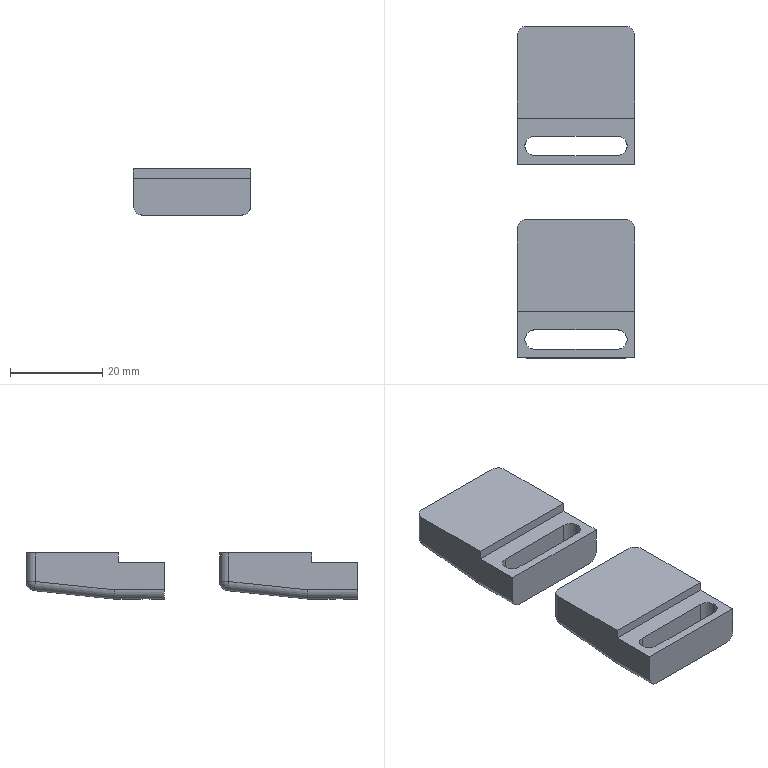NC program | NX | posted with a generic post | part box 25.5 x 72 x 10 mm
Lines 86 to 1188 of 60534:
(FIXED_CONTOUR , TOOL : D4R0.5)
N164 T16 M6
N166 G54
N168 G17 G0 G90 X3.812 Y-11.316 B0. C0. S9500 M3
N170 G43 Z30. H16
N172 Z1.2
N174 G94 G1 Z-4.301 F1000.
N176 G3 X4.012 Y-10.97 R0.4
N178 G1 Y-10.947 Z-4.21 F2500.
N180 X4.01 Y-10.907 Z-4.201
N182 X4.005 Y-10.808
N184 X4.003 Y-1.71
N186 X4.007 Y-1.464
N188 X4.012 Y-1.388 Z-4.189
N190 Y-1.294 Z-4.213
N192 Y-1.388 Z-4.189
N194 X4.011 Y-1.413 Z-4.193
N196 Y-1.541 Z-4.157
N198 Y-1.937 Z-4.103
N200 Y-2.334 Z-4.104
N202 Y-2.755 Z-4.101
N204 Y-7.911 Z-4.121
N206 Y-9.101 Z-4.128
N208 Y-10.709 Z-4.126
N210 Y-10.75 Z-4.132
N212 Y-10.808 Z-4.135
N214 Y-10.907 Z-4.19
N216 Y-10.919 Z-4.204
N218 X4.012 Y-10.947 Z-4.21
N220 Y-10.97 Z-4.301
N222 X4.018 Y-11.032
N224 Y-11.009 Z-4.209
N226 Y-10.907 Z-4.095
N228 Y-10.808 Z-4.039
N230 Y-10.789 Z-4.038
N232 Y-10.709 Z-4.026
N234 Y-8.924 Z-4.028
N236 Y-4.165 Z-4.013
N238 Y-2.926 Z-4.011
N240 Y-2.578 Z-4.02
N242 Y-2.084 Z-4.018
N244 Y-1.687 Z-4.072
N246 Y-1.388 Z-4.157
N248 Y-1.264 Z-4.189
N250 X4.023 Y-1.237 Z-4.167
N252 X4.028 Y-1.224 Z-4.157
N254 Y-1.388 Z-4.114
N256 Y-1.478 Z-4.086
N258 Y-1.785 Z-3.999
N260 Y-1.875 Z-3.979
N262 Y-2.181 Z-3.937
N264 Y-2.271 Z-3.935
N266 Y-2.703 Z-3.936
N268 Y-3.144 Z-3.94
N270 Y-7.903 Z-3.945
N272 Y-9.152 Z-3.947
N274 Y-10.709 Z-3.944
N276 Y-10.808 Z-3.95
N278 Y-10.907 Z-3.982
N280 Y-10.921 Z-3.991
N282 Y-10.942 Z-4.013
N284 Y-11.116 Z-4.208
N286 Y-11.139 Z-4.301
N288 X4.037 Y-11.246
N290 Y-11.223 Z-4.206
N292 Y-11.149 Z-4.123
N294 Y-11. Z-3.973
N296 Y-10.907 Z-3.912
N298 Y-10.808 Z-3.88
N300 Y-10.709 Z-3.874
N302 Y-4.958 Z-3.886
N304 Y-2.46 Z-3.878
N306 Y-2.181 Z-3.885
N308 Y-2.064 Z-3.901
N310 Y-1.785 Z-3.964
N312 Y-1.667 Z-3.998
N314 Y-1.388 Z-4.083
N316 Y-1.195 Z-4.136
N318 X4.049 Y-1.164 Z-4.113
N320 Y-1.346 Z-4.063
N322 Y-1.444 Z-4.032
N324 Y-1.841 Z-3.911
N326 Y-2.21 Z-3.828
N328 Y-2.238 Z-3.825
N330 Y-2.656 Z-3.816
N332 Y-2.975 Z-3.822
N334 Y-5.354 Z-3.827
N336 Y-7.338 Z-3.825
N338 Y-8.657 Z-3.824
N340 Y-10.709 Z-3.819
N342 Y-10.808 Z-3.821
N344 Y-10.907 Z-3.843
N346 Y-10.984 Z-3.877
N348 Y-11.097 Z-3.951
N350 Y-11.304 Z-4.159
N352 Y-11.328 Z-4.205
N354 Y-11.339 Z-4.301
N356 X4.063 Y-11.411
N358 Y-11.4 Z-4.206
N360 Y-11.38 Z-4.161
N362 Y-11.304 Z-4.019
N364 Y-11.211 Z-3.925
N366 Y-11.16 Z-3.891
N368 Y-10.907 Z-3.779
N370 Y-10.808 Z-3.758
N372 Y-10.709 Z-3.755
N374 Y-8.021 Z-3.763
N376 Y-6.257 Z-3.758
N378 Y-3.481 Z-3.756
N380 Y-2.975 Z-3.755
N382 Y-2.844 Z-3.753
N384 Y-2.578 Z-3.755
N386 Y-2.373 Z-3.761
N388 Y-2.277 Z-3.769
N390 Y-2.181 Z-3.788
N392 Y-1.976 Z-3.834
N394 Y-1.58 Z-3.955
N396 Y-1.388 Z-4.019
N398 Y-1.245 Z-4.063
N400 Y-1.135 Z-4.094
N402 X4.079 Y-1.1 Z-4.07
N404 Y-1.388 Z-3.981
N406 Y-1.785 Z-3.85
N408 Y-2.135 Z-3.745
N410 Y-2.357 Z-3.699
N412 Y-2.532 Z-3.684
N414 Y-2.744 Z-3.681
N416 Y-2.975 Z-3.686
N418 Y-6.978 Z-3.691
N420 Y-8.131 Z-3.696
N422 Y-10.709 Z-3.688
N424 Y-10.816 Z-3.692
N426 Y-10.916 Z-3.709
N428 Y-10.936 Z-3.716
N430 Y-11.304 Z-3.878
N432 Y-11.333 Z-3.909
N434 Y-11.447 Z-4.122
N436 Y-11.485 Z-4.207
N438 Y-11.496 Z-4.301
N440 X4.098 Y-11.595
N442 Y-11.584 Z-4.207
N444 Y-11.525 Z-4.077
N446 Y-11.446 Z-3.929
N448 Y-11.304 Z-3.783
N450 Y-11.217 Z-3.744
N452 Y-11.003 Z-3.67
N454 Y-10.907 Z-3.642
N456 Y-10.808 Z-3.626
N458 Y-10.709 Z-3.624
N460 Y-8.131 Z-3.63
N462 Y-6.4 Z-3.626
N464 Y-2.975 Z-3.621
N466 Y-2.674 Z-3.615
N468 Y-2.578 Z-3.619
N470 Y-2.436 Z-3.631
N472 Y-2.295 Z-3.66
N474 Y-2.181 Z-3.688
N476 Y-1.898 Z-3.773
N478 Y-1.785 Z-3.814
N480 Y-1.445 Z-3.927
N482 Y-1.388 Z-3.949
N484 Y-1.064 Z-4.049
N486 X4.117 Y-1.03 Z-4.03
N488 Y-1.388 Z-3.919
N490 Y-1.521 Z-3.869
N492 Y-1.785 Z-3.781
N494 Y-2.05 Z-3.686
N496 Y-2.181 Z-3.646
N498 Y-2.446 Z-3.581
N500 Y-2.512 Z-3.568
N502 Y-2.578 Z-3.562
N504 Y-2.802 Z-3.553
N506 Y-2.975 Z-3.557
N508 Y-8.527 Z-3.563
N510 Y-10.709 Z-3.559
N512 Y-10.808 Z-3.562
N514 Y-10.907 Z-3.577
N516 Y-11.09 Z-3.632
N518 Y-11.304 Z-3.705
N520 Y-11.357 Z-3.742
N522 Y-11.395 Z-3.772
N524 Y-11.445 Z-3.832
N526 Y-11.559 Z-3.949
N528 Y-11.603 Z-4.031
N530 Y-11.683 Z-4.208
N532 Y-11.694 Z-4.301
N534 X4.138 Y-11.765
N536 Y-11.758 Z-4.212
N538 Y-11.7 Z-4.011
N540 Y-11.682 Z-3.971
N542 Y-11.667 Z-3.956
N544 Y-11.538 Z-3.803
N546 Y-11.441 Z-3.724
N548 Y-11.304 Z-3.63
N550 Y-11.185 Z-3.589
N552 Y-10.907 Z-3.507
N554 Y-10.808 Z-3.492
N556 Y-10.709 Z-3.489
N558 Y-6.12 Z-3.492
N560 Y-2.941 Z-3.486
N562 Y-2.598 Z-3.501
N564 Y-2.578 Z-3.504
N566 Y-2.214 Z-3.594
N568 Y-2.149 Z-3.615
N570 Y-1.785 Z-3.746
N572 Y-1.603 Z-3.806
N574 Y-1.388 Z-3.888
N576 Y-0.992 Z-4.009
N578 X4.16 Y-0.953 Z-3.99
N580 Y-0.992 Z-3.981
N582 Y-1.176 Z-3.918
N584 Y-1.388 Z-3.853
N586 Y-1.692 Z-3.738
N588 Y-1.785 Z-3.707
N590 Y-2.181 Z-3.563
N592 Y-2.393 Z-3.502
N594 Y-2.578 Z-3.456
N596 Y-2.711 Z-3.439
N598 Y-2.975 Z-3.426
N600 Y-6.148 Z-3.43
N602 Y-10.709 Z-3.429
N604 Y-10.808 Z-3.431
N606 Y-10.907 Z-3.443
N608 Y-11.227 Z-3.525
N610 Y-11.304 Z-3.549
N612 Y-11.532 Z-3.705
N614 Y-11.694 Z-3.837
N616 Y-11.7 Z-3.845
N618 Y-11.764 Z-3.975
N620 Y-11.834 Z-4.216
N622 Y-11.841 Z-4.301
N624 X4.189 Y-11.936
N626 Y-11.929 Z-4.221
N628 Y-11.859 Z-3.975
N630 Y-11.79 Z-3.837
N632 Y-11.768 Z-3.805
N634 Y-11.7 Z-3.723
N636 Y-11.648 Z-3.68
N638 Y-11.565 Z-3.624
N640 Y-11.387 Z-3.511
N642 Y-11.304 Z-3.466
N644 Y-11.107 Z-3.422
N646 Y-10.907 Z-3.37
N648 Y-10.808 Z-3.359
N650 Y-10.709 Z-3.357
N652 Y-8.392 Z-3.359
N654 Y-2.975 Z-3.355
N656 Y-2.854 Z-3.361
N658 Y-2.589 Z-3.395
N660 Y-2.181 Z-3.515
N662 Y-1.785 Z-3.661
N664 Y-1.388 Z-3.812
N666 Y-0.992 Z-3.948
N668 Y-0.904 Z-3.967
N670 X4.204 Y-0.879 Z-3.955
N672 X4.218 Y-0.862 Z-3.949
N674 Y-0.992 Z-3.915
N676 Y-1.388 Z-3.78
N678 Y-1.523 Z-3.724
N680 Y-1.785 Z-3.625
N682 Y-1.92 Z-3.57
N684 Y-2.181 Z-3.474
N686 Y-2.317 Z-3.428
N688 Y-2.578 Z-3.352
N690 Y-2.646 Z-3.334
N692 Y-2.713 Z-3.322
N694 Y-2.975 Z-3.286
N696 Y-7.734 Z-3.288
N698 Y-8.924 Z-3.29
N700 Y-10.722 Z-3.286
N702 Y-10.808 Z-3.288
N704 Y-10.916 Z-3.3
N706 Y-11.304 Z-3.386
N708 Y-11.482 Z-3.483
N710 Y-11.7 Z-3.621
N712 Y-11.738 Z-3.65
N714 Y-11.838 Z-3.77
N716 Y-11.883 Z-3.836
N718 Y-11.953 Z-3.975
N720 Y-12.025 Z-4.227
N722 Y-12.032 Z-4.301
N724 X4.237 Y-12.097 Z-4.3
N726 X4.248 Y-12.126 Z-4.301
N728 Y-12.122 Z-4.236
N730 Y-12.115 Z-4.197
N732 Y-12.052 Z-3.975
N734 Y-11.981 Z-3.835
N736 Y-11.911 Z-3.733
N738 Y-11.812 Z-3.615
N740 Y-11.7 Z-3.528
N742 Y-11.582 Z-3.453
N744 Y-11.384 Z-3.345
N746 Y-11.304 Z-3.315
N748 Y-11.224 Z-3.292
N750 Y-11.003 Z-3.244
N752 Y-10.907 Z-3.234
N754 Y-10.806 Z-3.22
N756 Y-10.709 Z-3.223
N758 Y-8.332 Z-3.224
N760 Y-5.153 Z-3.223
N762 Y-3.567
N764 Y-3.17 Z-3.222
N766 Y-2.975 Z-3.227
N768 Y-2.833 Z-3.246
N770 Y-2.705 Z-3.27
N772 Y-2.578 Z-3.303
N774 Y-2.436 Z-3.344
N776 Y-2.181 Z-3.432
N778 Y-2.04 Z-3.483
N780 Y-1.785 Z-3.587
N782 Y-1.643 Z-3.641
N784 Y-1.388 Z-3.746
N786 Y-1.19 Z-3.813
N788 Y-0.992 Z-3.887
N790 Y-0.884 Z-3.921
N792 Y-0.823 Z-3.936
N794 X4.278 Y-0.782 Z-3.924
N796 Y-0.992 Z-3.858
N798 Y-1.388 Z-3.712
N800 Y-2.161 Z-3.396
N802 Y-2.578 Z-3.253
N804 Y-2.766 Z-3.205
N806 Y-2.975 Z-3.167
N808 Y-3.371 Z-3.158
N810 Y-4.165 Z-3.161
N812 Y-8.131 Z-3.158
N814 Y-10.724
N816 Y-10.808 Z-3.159
N818 Y-10.907 Z-3.169
N820 Y-11.09 Z-3.188
N822 Y-11.123 Z-3.195
N824 Y-11.304 Z-3.247
N826 Y-11.485 Z-3.313
N828 Y-11.7 Z-3.434
N830 Y-11.886 Z-3.579
N832 Y-11.985 Z-3.695
N834 Y-12.08 Z-3.833
N836 Y-12.097 Z-3.867
N838 Y-12.169 Z-4.037
N840 Y-12.181 Z-4.077
N842 Y-12.209 Z-4.264
N844 Z-4.301
N846 X4.317 Y-12.3
N848 Y-12.299 Z-4.254
N850 Y-12.266 Z-4.046
N852 Y-12.233 Z-3.962
N854 Y-12.183 Z-3.848
N856 Y-12.097 Z-3.696
N858 Y-12.066 Z-3.651
N860 Y-12.035 Z-3.614
N862 Y-11.967 Z-3.544
N864 Y-11.768 Z-3.39
N866 Y-11.7 Z-3.342
N868 Y-11.57 Z-3.269
N870 Y-11.372 Z-3.198
N872 Y-11.304 Z-3.171
N874 Y-11.174 Z-3.134
N876 Y-11.037 Z-3.111
N878 Y-10.842 Z-3.091
N880 Y-10.511 Z-3.088
N882 Y-4.822
N884 Y-3.768
N886 Y-3.371 Z-3.087
N888 Y-3.111 Z-3.094
N890 Y-2.975 Z-3.106
N892 Y-2.844 Z-3.13
N894 Y-2.578 Z-3.2
N896 Y-2.317 Z-3.29
N898 Y-2.181 Z-3.342
N900 Y-1.921 Z-3.448
N902 Y-1.785 Z-3.507
N904 Y-1.524 Z-3.614
N906 Y-1.388 Z-3.674
N908 Y-1.128 Z-3.771
N910 Y-0.992 Z-3.826
N912 Y-0.73 Z-3.91
N914 X4.358 Y-0.677 Z-3.897
N916 Y-0.992 Z-3.794
N918 Y-1.289 Z-3.674
N920 Y-1.388 Z-3.637
N922 Y-1.686 Z-3.506
N924 Y-1.785 Z-3.465
N926 Y-2.083 Z-3.335
N928 Y-2.181 Z-3.295
N930 Y-2.479 Z-3.181
N932 Y-2.578 Z-3.147
N934 Y-2.925 Z-3.055
N936 Y-2.975 Z-3.045
N938 Y-3.272 Z-3.018
N940 Y-3.371 Z-3.016
N942 Y-10.511
N944 Y-10.882 Z-3.023
N946 Y-10.957 Z-3.03
N948 Y-11.254 Z-3.081
N950 Y-11.304 Z-3.095
N952 Y-11.453 Z-3.154
N954 Y-11.651 Z-3.223
N956 Y-11.7 Z-3.251
N958 Y-11.849 Z-3.357
N960 Y-12.048 Z-3.509
N962 Y-12.097 Z-3.56
N964 Y-12.144 Z-3.62
N966 Y-12.167 Z-3.653
N968 Y-12.19 Z-3.696
N970 Y-12.286 Z-3.866
N972 Y-12.336 Z-3.983
N974 Y-12.354 Z-4.034
N976 Y-12.389 Z-4.247
N978 Y-12.392 Z-4.301
N980 X4.398 Y-12.483
N982 Y-12.477 Z-4.228
N984 Y-12.441 Z-4.022
N986 Y-12.406 Z-3.923
N988 Y-12.389 Z-3.884
N990 Y-12.34 Z-3.798
N992 Y-12.281 Z-3.685
N994 Y-12.221 Z-3.598
N996 Y-12.124 Z-3.479
N998 Y-12.097 Z-3.451
N1000 Y-11.93 Z-3.323
N1002 Y-11.763 Z-3.204
N1004 Y-11.7 Z-3.167
N1006 Y-11.534 Z-3.11
N1008 Y-11.367 Z-3.044
N1010 Y-11.304 Z-3.024
N1012 Y-10.97 Z-2.967
N1014 Y-10.907 Z-2.957
N1016 Y-10.511 Z-2.949
N1018 Y-3.371
N1020 Y-3.006 Z-2.983
N1022 Y-2.975 Z-2.989
N1024 Y-2.61 Z-3.087
N1026 Y-2.578 Z-3.098
N1028 Y-2.244 Z-3.225
N1030 Y-2.181 Z-3.251
N1032 Y-1.848 Z-3.396
N1034 Y-1.388 Z-3.602
N1036 Y-1.054 Z-3.736
N1038 Y-0.992 Z-3.763
N1040 Y-0.66 Z-3.875
N1042 Y-0.625 Z-3.885
N1044 X4.441 Y-0.575 Z-3.876
N1046 Y-0.676 Z-3.845
N1048 Y-0.816 Z-3.798
N1050 Y-0.992 Z-3.734
N1052 Y-1.223 Z-3.635
N1054 Y-1.388 Z-3.569
N1056 Y-1.619 Z-3.461
N1058 Y-1.785 Z-3.388
N1060 Y-2.016 Z-3.281
N1062 Y-2.181 Z-3.209
N1064 Y-2.412 Z-3.114
N1066 Y-2.578 Z-3.051
N1068 Y-2.694 Z-3.012
N1070 Y-2.975 Z-2.937
N1072 Y-3.09 Z-2.914
N1074 Y-3.371 Z-2.888
N1076 Y-10.511
N1078 Y-10.907 Z-2.895
N1080 Y-11.023 Z-2.915
N1082 Y-11.138 Z-2.929
N1084 Y-11.304 Z-2.958
N1086 Y-11.419 Z-2.997
N1088 Y-11.535 Z-3.031
N1090 Y-11.618 Z-3.064
N1092 Y-11.7 Z-3.093
N1094 Y-11.816 Z-3.159
N1096 Y-11.931 Z-3.229
N1098 Y-12.014 Z-3.288
N1100 Y-12.097 Z-3.352
N1102 Y-12.197 Z-3.454
N1104 Y-12.24 Z-3.5
N1106 Y-12.3 Z-3.576
N1108 Y-12.399 Z-3.718
N1110 Y-12.495 Z-3.902
N1112 Y-12.526 Z-4.004
N1114 Y-12.548 Z-4.159
N1116 Y-12.562 Z-4.232
N1118 Y-12.566 Z-4.301
N1120 X4.485 Y-12.652
N1122 Y-12.648 Z-4.223
N1124 Y-12.616 Z-4.059
N1126 Y-12.604 Z-3.979
N1128 Y-12.582 Z-3.916
N1130 Y-12.567 Z-3.865
N1132 Y-12.519 Z-3.753
N1134 Y-12.494 Z-3.71
N1136 Y-12.384 Z-3.552
N1138 Y-12.35 Z-3.509
N1140 Y-12.274 Z-3.427
N1142 Y-12.097 Z-3.249
N1144 Y-11.904 Z-3.132
N1146 Y-11.7 Z-3.015
N1148 Y-11.508 Z-2.958
N1150 Y-11.304 Z-2.889
N1152 Y-11.111 Z-2.866
N1154 Y-10.907 Z-2.831
N1156 Y-10.511 Z-2.823
N1158 Y-5.349 Z-2.826
N1160 Y-3.768 Z-2.824
N1162 Y-3.371 Z-2.825
N1164 Y-3.173 Z-2.844
N1166 Y-2.978 Z-2.882
N1168 Y-2.779 Z-2.935
N1170 Y-2.581 Z-3.001
N1172 Y-2.187 Z-3.162
N1174 Y-1.382 Z-3.537
N1176 Y-0.992 Z-3.705
N1178 Y-0.595 Z-3.845
N1180 Y-0.524 Z-3.867
N1182 X4.532 Y-0.473 Z-3.862
N1184 Y-0.595 Z-3.823
N1186 Y-0.694 Z-3.783
N1188 Y-0.992 Z-3.678
N1190 Y-1.289 Z-3.55
N1192 Y-1.388 Z-3.503
N1194 Y-1.487 Z-3.453
N1196 Y-1.785 Z-3.314
N1198 Y-1.884 Z-3.263
N1200 Y-2.28 Z-3.081
N1202 Y-2.578 Z-2.959
N1204 Y-2.627 Z-2.941
N1206 Y-2.826 Z-2.875
N1208 Y-3.024 Z-2.824
N1210 Y-3.173 Z-2.795
N1212 Y-3.272 Z-2.777
N1214 Y-3.371 Z-2.768
N1216 Y-8.652
N1218 Y-10.609
N1220 Y-10.907 Z-2.774
N1222 Y-10.957 Z-2.778
N1224 Y-11.105 Z-2.796
N1226 Y-11.204 Z-2.813
N1228 Y-11.304 Z-2.825
N1230 Y-11.502 Z-2.882
N1232 Y-11.601 Z-2.916
N1234 Y-11.7 Z-2.946
N1236 Y-11.898 Z-3.046
N1238 Y-11.998 Z-3.103
N1240 Y-12.097 Z-3.163
N1242 Y-12.196 Z-3.243
N1244 Y-12.248 Z-3.291
N1246 Y-12.355 Z-3.399
N1248 Y-12.472 Z-3.527
N1250 Y-12.494 Z-3.558
N1252 Y-12.572 Z-3.682
N1254 Y-12.627 Z-3.789
N1256 Y-12.643 Z-3.826
N1258 Y-12.688 Z-3.954
N1260 Y-12.733 Z-4.218
N1262 Y-12.737 Z-4.301
N1264 X4.582 Y-12.82
N1266 Y-12.817 Z-4.219
N1268 Y-12.771 Z-3.952
N1270 Y-12.725 Z-3.807
N1272 Y-12.667 Z-3.68
N1274 Y-12.639 Z-3.628
N1276 Y-12.613 Z-3.586
N1278 Y-12.494 Z-3.425
N1280 Y-12.401 Z-3.328
N1282 Y-12.296 Z-3.232
N1284 Y-12.097 Z-3.072
N1286 Y-11.8 Z-2.92
N1288 Y-11.7 Z-2.872
N1290 Y-11.303 Z-2.757
N1292 Y-11.007 Z-2.72
N1294 Y-10.907 Z-2.714
N1296 Y-10.511 Z-2.707
N1298 Y-3.371 Z-2.708
N1300 Y-3.173 Z-2.742
N1302 Y-3.074 Z-2.761
N1304 Y-2.975 Z-2.785
N1306 Y-2.876 Z-2.812
N1308 Y-2.677 Z-2.876
N1310 Y-2.578 Z-2.913
N1312 Y-2.38 Z-2.994
N1314 Y-2.181 Z-3.083
N1316 Y-1.984 Z-3.175
N1318 Y-1.785 Z-3.276
N1320 Y-1.587 Z-3.368
N1322 Y-1.388 Z-3.47
N1324 Y-1.189 Z-3.565
N1326 Y-0.992 Z-3.649
N1328 Y-0.794 Z-3.719
N1330 Y-0.595 Z-3.799
N1332 Y-0.419 Z-3.857
N1334 X4.634 Y-0.367 Z-3.85
N1336 Y-0.595 Z-3.775
N1338 Y-0.897 Z-3.653
N1340 Y-0.992 Z-3.62
N1342 Y-1.086 Z-3.579
N1344 Y-1.388 Z-3.436
N1346 Y-1.69 Z-3.281
N1348 Y-1.785 Z-3.237
N1350 Y-2.087 Z-3.083
N1352 Y-2.483 Z-2.904
N1354 Y-2.578 Z-2.865
N1356 Y-2.729 Z-2.809
N1358 Y-2.927 Z-2.746
N1360 Y-3.126 Z-2.697
N1362 Y-3.371 Z-2.653
N1364 Y-3.578 Z-2.645
N1366 Y-10.511
N1368 Y-10.907 Z-2.651
N1370 Y-11.058 Z-2.661
N1372 Y-11.2 Z-2.678
N1374 Y-11.304 Z-2.695
N1376 Y-11.407 Z-2.719
N1378 Y-11.7 Z-2.804
N1380 Y-11.804 Z-2.845
N1382 Y-12.097 Z-2.993
N1384 Y-12.201 Z-3.061
N1386 Y-12.399 Z-3.221
N1388 Y-12.494 Z-3.307
N1390 Y-12.532 Z-3.35
N1392 Y-12.674 Z-3.538
N1394 Y-12.717 Z-3.605
N1396 Y-12.811 Z-3.807
N1398 Y-12.857 Z-3.952
N1400 Y-12.899 Z-4.196
N1402 Y-12.902 Z-4.225
N1404 Y-12.906 Z-4.301
N1406 X4.683 Y-12.984 Z-4.3
N1408 Y-12.982 Z-4.249
N1410 Y-12.96 Z-4.041
N1412 Y-12.938 Z-3.954
N1414 Y-12.89 Z-3.799
N1416 Y-12.796 Z-3.599
N1418 Y-12.697 Z-3.445
N1420 Y-12.622 Z-3.346
N1422 Y-12.494 Z-3.207
N1424 Y-12.3 Z-3.051
N1426 Y-12.097 Z-2.917
N1428 Y-11.903 Z-2.82
N1430 Y-11.7 Z-2.74
N1432 Y-11.504 Z-2.682
N1434 Y-11.304 Z-2.636
N1436 Y-11.103 Z-2.604
N1438 Y-10.907 Z-2.591
N1440 Y-10.506 Z-2.586
N1442 Y-3.768 Z-2.585
N1444 Y-3.371 Z-2.601
N1446 Y-3.175 Z-2.635
N1448 Y-2.975 Z-2.683
N1450 Y-2.779 Z-2.745
N1452 Y-2.578 Z-2.819
N1454 Y-2.181 Z-2.997
N1456 Y-1.388 Z-3.403
N1458 Y-0.992 Z-3.592
N1460 Y-0.595 Z-3.752
N1462 Y-0.32 Z-3.843
N1464 X4.739 Y-0.27 Z-3.839
N1466 Y-0.537 Z-3.752
N1468 Y-0.595 Z-3.731
N1470 Y-0.711 Z-3.679
N1472 Y-0.992 Z-3.566
N1474 Y-1.108 Z-3.506
N1476 Y-1.388 Z-3.373
N1478 Y-1.504 Z-3.308
N1480 Y-1.785 Z-3.164
N1482 Y-1.901 Z-3.1
N1484 Y-2.181 Z-2.958
N1486 Y-2.298 Z-2.902
N1488 Y-2.578 Z-2.776
N1490 Y-2.834 Z-2.682
N1492 Y-2.975 Z-2.638
N1494 Y-3.231 Z-2.577
N1496 Y-3.371 Z-2.553
N1498 Y-3.487 Z-2.544
N1500 Y-3.768 Z-2.533
N1502 Y-6.941
N1504 Y-10.511
N1506 Y-10.907 Z-2.538
N1508 Y-11.047 Z-2.547
N1510 Y-11.164 Z-2.558
N1512 Y-11.304 Z-2.58
N1514 Y-11.56 Z-2.639
N1516 Y-11.7 Z-2.68
N1518 Y-11.817 Z-2.723
N1520 Y-12.015 Z-2.801
N1522 Y-12.097 Z-2.843
N1524 Y-12.353 Z-3.009
N1526 Y-12.412 Z-3.049
N1528 Y-12.494 Z-3.115
N1530 Y-12.61 Z-3.234
N1532 Y-12.698 Z-3.33
N1534 Y-12.808 Z-3.477
N1536 Y-12.89 Z-3.607
N1538 Y-12.903 Z-3.632
N1540 Y-12.975 Z-3.826
N1542 Y-13.01 Z-3.941
N1544 Y-13.034 Z-4.034
N1546 Y-13.057 Z-4.247
N1548 Y-13.059 Z-4.301
N1550 X4.799 Y-13.139
N1552 Y-13.137 Z-4.244
N1554 Y-13.112 Z-4.026
N1556 Y-13.088 Z-3.928
N1558 Y-13.062 Z-3.845
N1560 Y-12.993 Z-3.656
N1562 Y-12.909 Z-3.49
N1564 Y-12.89 Z-3.461
N1566 Y-12.779 Z-3.313
N1568 Y-12.65 Z-3.176
N1570 Y-12.518 Z-3.044
N1572 Y-12.494 Z-3.022
N1574 Y-12.332 Z-2.914
N1576 Y-12.17 Z-2.81
N1578 Y-12.097 Z-2.767
N1580 Y-11.935 Z-2.704
N1582 Y-11.7 Z-2.617
N1584 Y-11.62 Z-2.593
N1586 Y-11.304 Z-2.521
N1588 Y-11.223 Z-2.508
N1590 Y-10.988 Z-2.486
N1592 Y-10.907 Z-2.481
N1594 Y-10.511 Z-2.476
N1596 Y-6.148 Z-2.477
N1598 Y-4.796 Z-2.478
N1600 Y-3.768 Z-2.476
N1602 Y-3.606 Z-2.483
N1604 Y-3.371 Z-2.501
N1606 Y-3.29 Z-2.515
N1608 Y-2.975 Z-2.59
N1610 Y-2.894 Z-2.615
N1612 Y-2.578 Z-2.73
N1614 Y-2.416 Z-2.803
N1616 Y-2.181 Z-2.916
N1618 Y-2.02 Z-2.998
N1620 Y-1.785 Z-3.126
N1622 Y-1.623 Z-3.209
N1624 Y-1.388 Z-3.34
N1626 Y-1.226 Z-3.417
N1628 Y-0.992 Z-3.538
N1630 Y-0.83 Z-3.603
N1632 Y-0.595 Z-3.709
N1634 Y-0.477 Z-3.752
N1636 Y-0.216 Z-3.836
N1638 X4.858 Y-0.172 Z-3.832
N1640 Y-0.418 Z-3.752
N1642 Y-0.595 Z-3.686
N1644 Y-0.949 Z-3.528
N1646 Y-0.992 Z-3.511
N1648 Y-1.345 Z-3.329
N1650 Y-1.388 Z-3.308
N1652 Y-1.742 Z-3.111
N1654 Y-2.181 Z-2.873
N1656 Y-2.578 Z-2.685
N1658 Y-2.975 Z-2.541
N1660 Y-3.371 Z-2.45
N1662 Y-3.725 Z-2.422
N1664 Y-3.768 Z-2.42
N1666 Y-5.397 Z-2.424
N1668 Y-7.734 Z-2.419
N1670 Y-10.511 Z-2.42
N1672 Y-10.929 Z-2.426
N1674 Y-11.282 Z-2.458
N1676 Y-11.304 Z-2.462
N1678 Y-11.679 Z-2.546
N1680 Y-11.7 Z-2.553
N1682 Y-12.097 Z-2.701
N1684 Y-12.408 Z-2.883
N1686 Y-12.494 Z-2.939
N1688 Y-12.649 Z-3.077
N1690 Y-12.861 Z-3.295
N1692 Y-12.89 Z-3.335
N1694 Y-12.968 Z-3.457
N1696 Y-12.994 Z-3.503
N1698 Y-13.082 Z-3.68
N1700 Y-13.149 Z-3.864
N1702 Y-13.173 Z-3.945
N1704 Y-13.191 Z-4.019
N1706 Y-13.217 Z-4.242
N1708 Y-13.22 Z-4.301
N1710 X4.919 Y-13.299
N1712 Y-13.296 Z-4.24
N1714 Y-13.27 Z-4.011
N1716 Y-13.238 Z-3.883
N1718 Y-13.173 Z-3.705
N1720 Y-13.074 Z-3.505
N1722 Y-13.028 Z-3.424
N1724 Y-12.948 Z-3.298
N1726 Y-12.929 Z-3.271
N1728 Y-12.89 Z-3.224
N1730 Y-12.769 Z-3.1
N1732 Y-12.571 Z-2.923
N1734 Y-12.532 Z-2.89
N1736 Y-12.494 Z-2.865
N1738 Y-12.174 Z-2.678
N1740 Y-12.136 Z-2.657
N1742 Y-12.097 Z-2.64
N1744 Y-11.739 Z-2.508
N1746 Y-11.7 Z-2.497
N1748 Y-11.381 Z-2.425
N1750 Y-11.304 Z-2.41
N1752 Y-10.907 Z-2.374
N1754 Y-10.511 Z-2.369
N1756 Y-6.544 Z-2.37
N1758 Y-5.277 Z-2.373
N1760 Y-3.768 Z-2.37
N1762 Y-3.41 Z-2.398
N1764 Y-3.371 Z-2.404
N1766 Y-3.013 Z-2.486
N1768 Y-2.936 Z-2.51
N1770 Y-2.617 Z-2.626
N1772 Y-2.539 Z-2.661
N1774 Y-2.22 Z-2.814
N1776 Y-1.862 Z-3.009
N1778 Y-1.785 Z-3.054
N1780 Y-1.465 Z-3.233
N1782 Y-1.388 Z-3.279
N1784 Y-1.069 Z-3.443
N1786 Y-0.992 Z-3.486
N1788 Y-0.672 Z-3.629
N1790 Y-0.595 Z-3.666
N1792 Y-0.358 Z-3.755
N1794 Y-0.183 Z-3.813
N1796 Y-0.129 Z-3.829
N1798 X4.981 Y-0.085 Z-3.828
N1800 Y-0.296 Z-3.761
N1802 Y-0.595 Z-3.646
N1804 Y-0.796 Z-3.55
N1806 Y-0.992 Z-3.462
N1808 Y-1.192 Z-3.351
N1810 Y-1.388 Z-3.25
N1812 Y-1.589 Z-3.13
N1814 Y-1.785 Z-3.021
N1816 Y-1.986 Z-2.904
N1818 Y-2.282 Z-2.743
N1820 Y-2.578 Z-2.602
N1822 Y-2.678 Z-2.56
N1824 Y-2.874 Z-2.489
N1826 Y-2.975 Z-2.455
N1828 Y-3.075 Z-2.427
N1830 Y-3.271 Z-2.381
N1832 Y-3.371 Z-2.36
N1834 Y-3.472 Z-2.346
N1836 Y-3.768 Z-2.323
N1838 Y-4.958 Z-2.324
N1840 Y-10.511 Z-2.322
N1842 Y-10.907 Z-2.326
N1844 Y-11.304 Z-2.36
N1846 Y-11.505 Z-2.399
N1848 Y-11.7 Z-2.444
N1850 Y-11.801 Z-2.472
N1852 Y-12.097 Z-2.58
N1854 Y-12.197 Z-2.624
N1856 Y-12.363 Z-2.718
N1858 Y-12.494 Z-2.795
N1860 Y-12.594 Z-2.86
N1862 Y-12.76 Z-3.003
N1864 Y-12.893 Z-3.124
N1866 Y-12.991 Z-3.242
N1868 Y-13.041 Z-3.313
N1870 Y-13.09 Z-3.39
N1872 Y-13.156 Z-3.508
N1874 Y-13.269 Z-3.739
N1876 Y-13.287 Z-3.788
N1878 Y-13.319 Z-3.895
N1880 Y-13.342 Z-4.011
N1882 Y-13.366 Z-4.24
N1884 Y-13.367 Z-4.301
N1886 X5.046 Y-13.44
N1888 Y-13.439 Z-4.24
N1890 Y-13.415 Z-4.013
N1892 Y-13.392 Z-3.898
N1894 Y-13.344 Z-3.738
N1896 Y-13.287 Z-3.6
N1898 Y-13.243 Z-3.51
N1900 Y-13.155 Z-3.355
N1902 Y-13.055 Z-3.211
N1904 Y-13.022 Z-3.171
N1906 Y-12.89 Z-3.028
N1908 Y-12.824 Z-2.969
N1910 Y-12.659 Z-2.828
N1912 Y-12.494 Z-2.721
N1914 Y-12.262 Z-2.591
N1916 Y-12.097 Z-2.518
N1918 Y-11.866 Z-2.435
N1920 Y-11.7 Z-2.388
N1922 Y-11.634 Z-2.373
N1924 Y-11.304 Z-2.309
N1926 Y-10.907 Z-2.276
N1928 Y-10.511 Z-2.272
N1930 Y-4.098
N1932 Y-3.768 Z-2.274
N1934 Y-3.536 Z-2.291
N1936 Y-3.371 Z-2.313
N1938 Y-3.14 Z-2.364
N1940 Y-2.975 Z-2.41
N1942 Y-2.743 Z-2.49
N1944 Y-2.578 Z-2.559
N1946 Y-2.347 Z-2.669
N1948 Y-2.115 Z-2.793
N1950 Y-1.718 Z-3.023
N1952 Y-1.388 Z-3.221
N1954 Y-1.322 Z-3.255
N1956 Y-0.992 Z-3.438
N1958 Y-0.925 Z-3.467
N1960 Y-0.595 Z-3.626
N1962 Y-0.232 Z-3.767
N1964 Y-0.039 Z-3.827
N1966 X5.043 Y0.005
N1968 X5.066 Y0.045
N1970 X5.106 Y0.065
N1972 Z0.373
N1974 G0 Z1.173
N1976 X4.032 Y1.259
N1978 Z0.373
N1980 G1 Z-4.213 F1000.
N1982 X4.009 Y1.268
N1984 X4.012 Y1.293
N1986 Y1.388 Z-4.189 F2500.
N1988 X4.007 Y1.464 Z-4.201
N1990 X4.003 Y1.75
N1992 X4.005 Y10.808
N1994 X4.01 Y10.907
N1996 X4.012 Y10.947 Z-4.21
N1998 Y10.97 Z-4.301
N2000 Y10.947 Z-4.21
N2002 X4.011 Y10.919 Z-4.204
N2004 Y10.907 Z-4.19
N2006 Y10.808 Z-4.135
N2008 Y10.75 Z-4.132
N2010 Y10.709 Z-4.126
N2012 Y7.118 Z-4.117
N2014 Y2.755 Z-4.101
N2016 Y2.181 Z-4.104
N2018 Y1.937 Z-4.103
N2020 Y1.541 Z-4.157
N2022 Y1.413 Z-4.193
N2024 X4.012 Y1.388 Z-4.189
N2026 Y1.293 Z-4.213
N2028 X4.018 Y1.263 Z-4.189
N2030 Y1.388 Z-4.157
N2032 Y1.687 Z-4.074
N2034 Y2.084 Z-4.018
N2036 Y2.578 Z-4.02
N2038 Y2.926 Z-4.011
N2040 Y5.751 Z-4.017
N2042 Y8.924 Z-4.026
N2044 Y10.709
N2046 Y10.789 Z-4.038
N2048 Y10.808 Z-4.039
N2050 Y10.907 Z-4.095
N2052 Y11.009 Z-4.209
N2054 Y11.032 Z-4.301
N2056 X4.028 Y11.139
N2058 Y11.116 Z-4.208
N2060 Y10.942 Z-4.013
N2062 Y10.921 Z-3.991
N2064 Y10.907 Z-3.982
N2066 Y10.808 Z-3.95
N2068 Y10.709 Z-3.944
N2070 Y7.734 Z-3.942
N2072 Y3.937 Z-3.937
N2074 Y2.975
N2076 Y2.703 Z-3.934
N2078 Y2.271
N2080 Y2.181 Z-3.936
N2082 Y1.875 Z-3.98
N2084 Y1.785 Z-4.001
N2086 Y1.478 Z-4.086
N2088 Y1.388 Z-4.114
N2090 Y1.223 Z-4.158
N2092 X4.037 Y1.195 Z-4.136
N2094 Y1.388 Z-4.083
N2096 Y1.667 Z-3.998
N2098 Y1.785 Z-3.965
N2100 Y2.064 Z-3.9
N2102 Y2.181 Z-3.883
N2104 Y2.46 Z-3.874
N2106 Y10.709
N2108 Y10.808 Z-3.88
N2110 Y10.907 Z-3.912
N2112 Y11. Z-3.973
N2114 Y11.149 Z-4.123
N2116 Y11.223 Z-4.206
N2118 Y11.246 Z-4.301
N2120 X4.043 Y11.305 Z-4.3
N2122 X4.049 Y11.339 Z-4.301
N2124 Y11.328 Z-4.205
N2126 Y11.304 Z-4.159
N2128 Y11.097 Z-3.951
N2130 Y10.984 Z-3.877
N2132 Y10.907 Z-3.843
N2134 Y10.808 Z-3.821
N2136 Y10.709 Z-3.818
N2138 Y7.734 Z-3.821
N2140 Y2.975 Z-3.817
N2142 Y2.578 Z-3.81
N2144 Y2.238 Z-3.822
N2146 Y2.21 Z-3.825
N2148 Y1.841 Z-3.911
N2150 Y1.444 Z-4.032
N2152 Y1.346 Z-4.064
N2154 Y1.164 Z-4.114
N2156 X4.063 Y1.135 Z-4.094
N2158 Y1.245 Z-4.063
N2160 Y1.388 Z-4.019
N2162 Y1.58 Z-3.955
N2164 Y1.976 Z-3.835
N2166 Y2.181 Z-3.786
N2168 Y2.277 Z-3.767
N2170 Y2.373 Z-3.757
N2172 Y2.578 Z-3.746
N2174 Y2.975 Z-3.751
N2176 Y6.148 Z-3.755
N2178 Y8.241 Z-3.761
N2180 Y10.709 Z-3.755
N2182 Y10.808 Z-3.758
N2184 Y10.907 Z-3.779
N2186 Y11.16 Z-3.891
N2188 Y11.211 Z-3.925
N2190 Y11.304 Z-4.019
N2192 Y11.38 Z-4.161
N2194 Y11.4 Z-4.206
N2196 Y11.411 Z-4.301
N2198 X4.079 Y11.496
N2200 Y11.485 Z-4.207
N2202 Y11.447 Z-4.122
N2204 Y11.333 Z-3.909
N2206 Y11.304 Z-3.878
N2208 Y10.936 Z-3.716
N2210 Y10.907 Z-3.707
N2212 Y10.808 Z-3.691
N2214 Y10.709 Z-3.688
N2216 Y8.131 Z-3.696
N2218 Y4.958 Z-3.685
N2220 Y2.975 Z-3.683
N2222 Y2.744 Z-3.677
N2224 Y2.578
N2226 Y2.532 Z-3.68
N2228 Y2.357 Z-3.698
N2230 Y2.135 Z-3.745
N2232 Y1.738 Z-3.865
N2234 Y1.388 Z-3.981
N2236 Y1.1 Z-4.07
N2238 X4.098 Y1.064 Z-4.049
N2240 Y1.388 Z-3.948
N2242 Y1.445 Z-3.927
N2244 Y1.785 Z-3.814
N2246 Y1.898 Z-3.773
N2248 Y2.181 Z-3.687
N2250 Y2.295 Z-3.66
N2252 Y2.436 Z-3.631
N2254 Y2.578 Z-3.616
N2256 Y2.674 Z-3.612
N2258 Y2.975 Z-3.619
N2260 Y6.148 Z-3.624
N2262 Y8.131 Z-3.629
N2264 Y10.709 Z-3.624
N2266 Y10.808 Z-3.626
N2268 Y10.907 Z-3.642
N2270 Y11.003 Z-3.67
N2272 Y11.217 Z-3.744
N2274 Y11.304 Z-3.783
N2276 Y11.446 Z-3.929
N2278 Y11.525 Z-4.077
N2280 Y11.584 Z-4.207
N2282 Y11.595 Z-4.301
N2284 X4.117 Y11.694
N2286 Y11.683 Z-4.208
N2288 Y11.603 Z-4.031
N2290 Y11.559 Z-3.949
N2292 Y11.445 Z-3.832
N2294 Y11.395 Z-3.772
N2296 Y11.357 Z-3.742
N2298 Y11.304 Z-3.705
N2300 Y11.09 Z-3.632
N2302 Y10.907 Z-3.577
N2304 Y10.808 Z-3.562
N2306 Y10.709 Z-3.559
N2308 Y7.734 Z-3.562
N2310 Y2.975 Z-3.555
N2312 Y2.802 Z-3.551
N2314 Y2.578 Z-3.561
N2316 Y2.512 Z-3.568
N2318 Y2.446 Z-3.581
N2320 Y2.181 Z-3.646
N2322 Y2.05 Z-3.686
N2324 Y1.785 Z-3.781
N2326 Y1.521 Z-3.869
N2328 Y1.388 Z-3.919
N2330 Y1.03 Z-4.03
N2332 X4.138 Y0.992 Z-4.009
N2334 Y1.388 Z-3.887
N2336 Y1.603 Z-3.807
N2338 Y1.785 Z-3.746
N2340 Y2.181 Z-3.602
N2342 Y2.214 Z-3.593
N2344 Y2.578 Z-3.504
N2346 Y2.757 Z-3.493
N2348 Y2.941 Z-3.485
N2350 Y6.176 Z-3.49
N2352 Y10.709 Z-3.489
N2354 Y10.808 Z-3.492
N2356 Y10.907 Z-3.507
N2358 Y11.185 Z-3.589
N2360 Y11.304 Z-3.63
N2362 Y11.441 Z-3.724